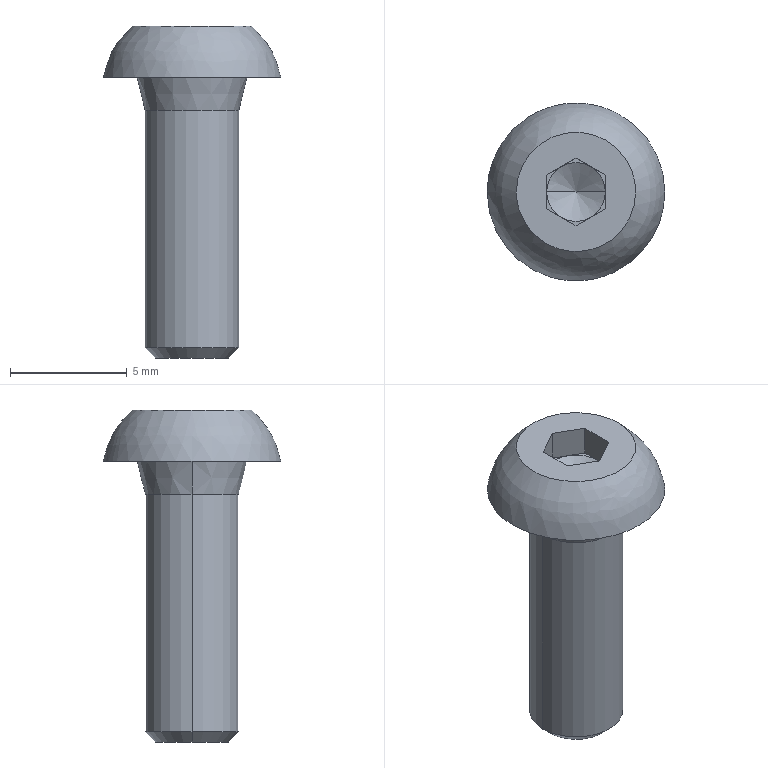Part | SolidWorks | features BaseBody 1 | 1 solid | 24 faces | box 7.6 x 7.6 x 14.2 mm | volume 222.779 mm3 | plane 15 | cone 6 | cylinder 2 | spline 1 | commonest cylinder face diameters 4 x2
STEP:
#1=CARTESIAN_POINT('',(2.,0.,-10.171));
#2=VERTEX_POINT('',#1);
#3=CARTESIAN_POINT('',(-2.,0.,-10.171));
#4=VERTEX_POINT('',#3);
#5=CARTESIAN_POINT('',(0.,0.,-10.171));
#6=DIRECTION('',(0.,0.,1.));
#7=DIRECTION('',(1.,0.,0.));
#8=AXIS2_PLACEMENT_3D('',#5,#6,#7);
#9=CIRCLE('',#8,2.);
#10=EDGE_CURVE('',#2,#4,#9,.T.);
#11=ORIENTED_EDGE('',*,*,#10,.T.);
#12=CARTESIAN_POINT('',(-2.,0.,0.));
#13=VERTEX_POINT('',#12);
#14=CARTESIAN_POINT('',(-2.,0.,-10.6));
#15=DIRECTION('',(0.,0.,1.));
#16=VECTOR('',#15,1000.);
#17=LINE('',#14,#16);
#18=EDGE_CURVE('',#4,#13,#17,.T.);
#19=ORIENTED_EDGE('',*,*,#18,.T.);
#20=CARTESIAN_POINT('',(2.,0.,0.));
#21=VERTEX_POINT('',#20);
#22=CARTESIAN_POINT('',(0.,0.,0.));
#23=DIRECTION('',(0.,0.,-1.));
#24=DIRECTION('',(1.,0.,0.));
#25=AXIS2_PLACEMENT_3D('',#22,#23,#24);
#26=CIRCLE('',#25,2.);
#27=EDGE_CURVE('',#13,#21,#26,.T.);
#28=ORIENTED_EDGE('',*,*,#27,.T.);
#29=CARTESIAN_POINT('',(2.,0.,-10.6));
#30=DIRECTION('',(0.,0.,1.));
#31=VECTOR('',#30,1000.);
#32=LINE('',#29,#31);
#33=EDGE_CURVE('',#2,#21,#32,.T.);
#34=ORIENTED_EDGE('',*,*,#33,.F.);
#35=EDGE_LOOP('',(#11,#19,#28,#34));
#36=FACE_OUTER_BOUND('',#35,.T.);
#37=CARTESIAN_POINT('',(0.,0.,-10.6));
#38=DIRECTION('',(0.,0.,1.));
#39=DIRECTION('',(1.,0.,0.));
#40=AXIS2_PLACEMENT_3D('',#37,#38,#39);
#41=CYLINDRICAL_SURFACE('',#40,2.);
#42=ADVANCED_FACE('',(#36),#41,.T.);
#43=ORIENTED_EDGE('',*,*,#27,.F.);
#44=CARTESIAN_POINT('',(-2.35,0.,1.4));
#45=VERTEX_POINT('',#44);
#46=CARTESIAN_POINT('',(-2.35,0.,1.4));
#47=DIRECTION('',(-0.2425,0.,0.9701));
#48=VECTOR('',#47,1000.);
#49=LINE('',#46,#48);
#50=EDGE_CURVE('',#13,#45,#49,.T.);
#51=ORIENTED_EDGE('',*,*,#50,.T.);
#52=CARTESIAN_POINT('',(2.35,0.,1.4));
#53=VERTEX_POINT('',#52);
#54=CARTESIAN_POINT('',(0.,0.,1.4));
#55=DIRECTION('',(0.,0.,-1.));
#56=DIRECTION('',(1.,0.,0.));
#57=AXIS2_PLACEMENT_3D('',#54,#55,#56);
#58=CIRCLE('',#57,2.35);
#59=EDGE_CURVE('',#45,#53,#58,.T.);
#60=ORIENTED_EDGE('',*,*,#59,.T.);
#61=CARTESIAN_POINT('',(2.35,0.,1.4));
#62=DIRECTION('',(0.2425,0.,0.9701));
#63=VECTOR('',#62,1000.);
#64=LINE('',#61,#63);
#65=EDGE_CURVE('',#21,#53,#64,.T.);
#66=ORIENTED_EDGE('',*,*,#65,.F.);
#67=EDGE_LOOP('',(#43,#51,#60,#66));
#68=FACE_OUTER_BOUND('',#67,.T.);
#69=CARTESIAN_POINT('',(0.,0.,1.4));
#70=DIRECTION('',(0.,0.,1.));
#71=DIRECTION('',(1.,0.,0.));
#72=AXIS2_PLACEMENT_3D('',#69,#70,#71);
#73=CONICAL_SURFACE('',#72,2.35,0.245);
#74=ADVANCED_FACE('',(#68),#73,.T.);
#75=CARTESIAN_POINT('',(1.571,0.,-10.6));
#76=VERTEX_POINT('',#75);
#77=CARTESIAN_POINT('',(-1.571,0.,-10.6));
#78=VERTEX_POINT('',#77);
#79=CARTESIAN_POINT('',(0.,0.,-10.6));
#80=DIRECTION('',(0.,0.,1.));
#81=DIRECTION('',(1.,0.,0.));
#82=AXIS2_PLACEMENT_3D('',#79,#80,#81);
#83=CIRCLE('',#82,1.571);
#84=EDGE_CURVE('',#76,#78,#83,.T.);
#85=ORIENTED_EDGE('',*,*,#84,.T.);
#86=CARTESIAN_POINT('',(-2.,0.,-10.171));
#87=DIRECTION('',(-0.7071,0.,0.7071));
#88=VECTOR('',#87,1000.);
#89=LINE('',#86,#88);
#90=EDGE_CURVE('',#78,#4,#89,.T.);
#91=ORIENTED_EDGE('',*,*,#90,.T.);
#92=ORIENTED_EDGE('',*,*,#10,.F.);
#93=CARTESIAN_POINT('',(2.,0.,-10.171));
#94=DIRECTION('',(0.7071,0.,0.7071));
#95=VECTOR('',#94,1000.);
#96=LINE('',#93,#95);
#97=EDGE_CURVE('',#76,#2,#96,.T.);
#98=ORIENTED_EDGE('',*,*,#97,.F.);
#99=EDGE_LOOP('',(#85,#91,#92,#98));
#100=FACE_OUTER_BOUND('',#99,.T.);
#101=CARTESIAN_POINT('',(0.,0.,-10.171));
#102=DIRECTION('',(0.,0.,1.));
#103=DIRECTION('',(1.,0.,0.));
#104=AXIS2_PLACEMENT_3D('',#101,#102,#103);
#105=CONICAL_SURFACE('',#104,2.,0.7854);
#106=ADVANCED_FACE('',(#100),#105,.T.);
#107=CARTESIAN_POINT('',(0.,0.,1.578));
#108=VERTEX_POINT('',#107);
#109=CARTESIAN_POINT('',(1.25,0.,2.3));
#110=VERTEX_POINT('',#109);
#111=CARTESIAN_POINT('',(1.25,0.,2.3));
#112=DIRECTION('',(0.866,0.,0.5));
#113=VECTOR('',#112,1000.);
#114=LINE('',#111,#113);
#115=EDGE_CURVE('',#108,#110,#114,.T.);
#116=ORIENTED_EDGE('',*,*,#115,.F.);
#117=CARTESIAN_POINT('',(-1.25,0.,2.3));
#118=VERTEX_POINT('',#117);
#119=CARTESIAN_POINT('',(-1.25,0.,2.3));
#120=DIRECTION('',(-0.866,0.,0.5));
#121=VECTOR('',#120,1000.);
#122=LINE('',#119,#121);
#123=EDGE_CURVE('',#108,#118,#122,.T.);
#124=ORIENTED_EDGE('',*,*,#123,.T.);
#125=CARTESIAN_POINT('',(-0.625,-1.083,2.3));
#126=VERTEX_POINT('',#125);
#127=CARTESIAN_POINT('',(0.,0.,2.3));
#128=DIRECTION('',(0.,0.,-1.));
#129=DIRECTION('',(1.,0.,0.));
#130=AXIS2_PLACEMENT_3D('',#127,#128,#129);
#131=CIRCLE('',#130,1.25);
#132=EDGE_CURVE('',#126,#118,#131,.T.);
#133=ORIENTED_EDGE('',*,*,#132,.F.);
#134=CARTESIAN_POINT('',(0.625,-1.083,2.3));
#135=VERTEX_POINT('',#134);
#136=CARTESIAN_POINT('',(0.,0.,2.3));
#137=DIRECTION('',(0.,0.,-1.));
#138=DIRECTION('',(1.,0.,0.));
#139=AXIS2_PLACEMENT_3D('',#136,#137,#138);
#140=CIRCLE('',#139,1.25);
#141=EDGE_CURVE('',#135,#126,#140,.T.);
#142=ORIENTED_EDGE('',*,*,#141,.F.);
#143=CARTESIAN_POINT('',(0.,0.,2.3));
#144=DIRECTION('',(0.,0.,-1.));
#145=DIRECTION('',(1.,0.,0.));
#146=AXIS2_PLACEMENT_3D('',#143,#144,#145);
#147=CIRCLE('',#146,1.25);
#148=EDGE_CURVE('',#110,#135,#147,.T.);
#149=ORIENTED_EDGE('',*,*,#148,.F.);
#150=EDGE_LOOP('',(#116,#124,#133,#142,#149));
#151=FACE_OUTER_BOUND('',#150,.T.);
#152=CARTESIAN_POINT('',(0.,0.,2.3));
#153=DIRECTION('',(0.,0.,1.));
#154=DIRECTION('',(1.,0.,0.));
#155=AXIS2_PLACEMENT_3D('',#152,#153,#154);
#156=CONICAL_SURFACE('',#155,1.25,1.047);
#157=ADVANCED_FACE('',(#151),#156,.F.);
#158=ORIENTED_EDGE('',*,*,#18,.F.);
#159=CARTESIAN_POINT('',(0.,0.,-10.171));
#160=DIRECTION('',(0.,0.,1.));
#161=DIRECTION('',(1.,0.,0.));
#162=AXIS2_PLACEMENT_3D('',#159,#160,#161);
#163=CIRCLE('',#162,2.);
#164=EDGE_CURVE('',#4,#2,#163,.T.);
#165=ORIENTED_EDGE('',*,*,#164,.T.);
#166=ORIENTED_EDGE('',*,*,#33,.T.);
#167=CARTESIAN_POINT('',(0.,0.,0.));
#168=DIRECTION('',(0.,0.,-1.));
#169=DIRECTION('',(1.,0.,0.));
#170=AXIS2_PLACEMENT_3D('',#167,#168,#169);
#171=CIRCLE('',#170,2.);
#172=EDGE_CURVE('',#21,#13,#171,.T.);
#173=ORIENTED_EDGE('',*,*,#172,.T.);
#174=EDGE_LOOP('',(#158,#165,#166,#173));
#175=FACE_OUTER_BOUND('',#174,.T.);
#176=CARTESIAN_POINT('',(0.,0.,-10.6));
#177=DIRECTION('',(0.,0.,1.));
#178=DIRECTION('',(1.,0.,0.));
#179=AXIS2_PLACEMENT_3D('',#176,#177,#178);
#180=CYLINDRICAL_SURFACE('',#179,2.);
#181=ADVANCED_FACE('',(#175),#180,.T.);
#182=ORIENTED_EDGE('',*,*,#50,.F.);
#183=ORIENTED_EDGE('',*,*,#172,.F.);
#184=ORIENTED_EDGE('',*,*,#65,.T.);
#185=CARTESIAN_POINT('',(0.,0.,1.4));
#186=DIRECTION('',(0.,0.,-1.));
#187=DIRECTION('',(1.,0.,0.));
#188=AXIS2_PLACEMENT_3D('',#185,#186,#187);
#189=CIRCLE('',#188,2.35);
#190=EDGE_CURVE('',#53,#45,#189,.T.);
#191=ORIENTED_EDGE('',*,*,#190,.T.);
#192=EDGE_LOOP('',(#182,#183,#184,#191));
#193=FACE_OUTER_BOUND('',#192,.T.);
#194=CARTESIAN_POINT('',(0.,0.,1.4));
#195=DIRECTION('',(0.,0.,1.));
#196=DIRECTION('',(1.,0.,0.));
#197=AXIS2_PLACEMENT_3D('',#194,#195,#196);
#198=CONICAL_SURFACE('',#197,2.35,0.245);
#199=ADVANCED_FACE('',(#193),#198,.T.);
#200=ORIENTED_EDGE('',*,*,#90,.F.);
#201=CARTESIAN_POINT('',(0.,0.,-10.6));
#202=DIRECTION('',(0.,0.,1.));
#203=DIRECTION('',(1.,0.,0.));
#204=AXIS2_PLACEMENT_3D('',#201,#202,#203);
#205=CIRCLE('',#204,1.571);
#206=EDGE_CURVE('',#78,#76,#205,.T.);
#207=ORIENTED_EDGE('',*,*,#206,.T.);
#208=ORIENTED_EDGE('',*,*,#97,.T.);
#209=ORIENTED_EDGE('',*,*,#164,.F.);
#210=EDGE_LOOP('',(#200,#207,#208,#209));
#211=FACE_OUTER_BOUND('',#210,.T.);
#212=CARTESIAN_POINT('',(0.,0.,-10.171));
#213=DIRECTION('',(0.,0.,1.));
#214=DIRECTION('',(1.,0.,0.));
#215=AXIS2_PLACEMENT_3D('',#212,#213,#214);
#216=CONICAL_SURFACE('',#215,2.,0.7854);
#217=ADVANCED_FACE('',(#211),#216,.T.);
#218=CARTESIAN_POINT('',(-3.8,0.,1.4));
#219=VERTEX_POINT('',#218);
#220=CARTESIAN_POINT('',(3.8,-0.001343,1.4));
#221=VERTEX_POINT('',#220);
#222=CARTESIAN_POINT('',(-3.8,0.,1.4));
#223=CARTESIAN_POINT('',(-3.8,-0.251,1.4));
#224=CARTESIAN_POINT('',(-3.775,-0.4979,1.4));
#225=CARTESIAN_POINT('',(-3.679,-0.9836,1.4));
#226=CARTESIAN_POINT('',(-3.606,-1.225,1.4));
#227=CARTESIAN_POINT('',(-3.415,-1.685,1.4));
#228=CARTESIAN_POINT('',(-3.298,-1.903,1.4));
#229=CARTESIAN_POINT('',(-3.023,-2.316,1.4));
#230=CARTESIAN_POINT('',(-2.862,-2.512,1.4));
#231=CARTESIAN_POINT('',(-2.511,-2.863,1.4));
#232=CARTESIAN_POINT('',(-2.32,-3.02,1.4));
#233=CARTESIAN_POINT('',(-1.905,-3.298,1.4));
#234=CARTESIAN_POINT('',(-1.684,-3.416,1.4));
#235=CARTESIAN_POINT('',(-1.226,-3.605,1.4));
#236=CARTESIAN_POINT('',(-0.9869,-3.678,1.4));
#237=CARTESIAN_POINT('',(-0.4964,-3.776,1.4));
#238=CARTESIAN_POINT('',(-0.2498,-3.8,1.4));
#239=CARTESIAN_POINT('',(0.2458,-3.8,1.4));
#240=CARTESIAN_POINT('',(0.4975,-3.775,1.4));
#241=CARTESIAN_POINT('',(0.9849,-3.679,1.4));
#242=CARTESIAN_POINT('',(1.222,-3.607,1.4));
#243=CARTESIAN_POINT('',(1.682,-3.417,1.4));
#244=CARTESIAN_POINT('',(1.904,-3.298,1.4));
#245=CARTESIAN_POINT('',(2.316,-3.023,1.4));
#246=CARTESIAN_POINT('',(2.508,-2.866,1.4));
#247=CARTESIAN_POINT('',(2.863,-2.511,1.4));
#248=CARTESIAN_POINT('',(3.021,-2.319,1.4));
#249=CARTESIAN_POINT('',(3.296,-1.907,1.4));
#250=CARTESIAN_POINT('',(3.415,-1.685,1.4));
#251=CARTESIAN_POINT('',(3.606,-1.225,1.4));
#252=CARTESIAN_POINT('',(3.678,-0.988,1.4));
#253=CARTESIAN_POINT('',(3.775,-0.5012,1.4));
#254=CARTESIAN_POINT('',(3.8,-0.2493,1.4));
#255=CARTESIAN_POINT('',(3.8,-0.001343,1.4));
#256=B_SPLINE_CURVE_WITH_KNOTS('',3,(#222,#223,#224,#225,#226,#227,#228,#229,#230,#231,#232,#233,#234,#235,#236,#237,#238,#239,#240,#241,#242,#243,#244,#245,#246,#247,#248,#249,#250,#251,#252,#253,#254,#255),.UNSPECIFIED.,.F.,.F.,(4,2,2,2,2,2,2,2,2,2,2,2,2,2,2,2,4),(0.,0.0007424,0.001485,0.002227,0.00297,0.003712,0.004455,0.005197,0.00594,0.006682,0.007424,0.008167,0.008909,0.009652,0.01039,0.01114,0.01188),.UNSPECIFIED.);
#257=EDGE_CURVE('',#219,#221,#256,.T.);
#258=ORIENTED_EDGE('',*,*,#257,.F.);
#259=CARTESIAN_POINT('',(3.8,-0.001343,1.4));
#260=CARTESIAN_POINT('',(3.8,0.2466,1.4));
#261=CARTESIAN_POINT('',(3.776,0.4931,1.4));
#262=CARTESIAN_POINT('',(3.679,0.9829,1.4));
#263=CARTESIAN_POINT('',(3.606,1.223,1.4));
#264=CARTESIAN_POINT('',(3.417,1.681,1.4));
#265=CARTESIAN_POINT('',(3.3,1.901,1.4));
#266=CARTESIAN_POINT('',(3.022,2.318,1.4));
#267=CARTESIAN_POINT('',(2.865,2.509,1.4));
#268=CARTESIAN_POINT('',(2.515,2.86,1.4));
#269=CARTESIAN_POINT('',(2.319,3.02,1.4));
#270=CARTESIAN_POINT('',(1.906,3.297,1.4));
#271=CARTESIAN_POINT('',(1.688,3.414,1.4));
#272=CARTESIAN_POINT('',(1.229,3.605,1.4));
#273=CARTESIAN_POINT('',(0.9869,3.678,1.4));
#274=CARTESIAN_POINT('',(0.5011,3.775,1.4));
#275=CARTESIAN_POINT('',(0.2544,3.8,1.4));
#276=CARTESIAN_POINT('',(-0.2467,3.8,1.4));
#277=CARTESIAN_POINT('',(-0.4947,3.776,1.4));
#278=CARTESIAN_POINT('',(-0.9803,3.68,1.4));
#279=CARTESIAN_POINT('',(-1.221,3.607,1.4));
#280=CARTESIAN_POINT('',(-1.682,3.417,1.4));
#281=CARTESIAN_POINT('',(-1.901,3.3,1.4));
#282=CARTESIAN_POINT('',(-2.313,3.025,1.4));
#283=CARTESIAN_POINT('',(-2.509,2.864,1.4));
#284=CARTESIAN_POINT('',(-2.86,2.514,1.4));
#285=CARTESIAN_POINT('',(-3.018,2.323,1.4));
#286=CARTESIAN_POINT('',(-3.296,1.908,1.4));
#287=CARTESIAN_POINT('',(-3.414,1.687,1.4));
#288=CARTESIAN_POINT('',(-3.604,1.229,1.4));
#289=CARTESIAN_POINT('',(-3.677,0.9912,1.4));
#290=CARTESIAN_POINT('',(-3.775,0.4995,1.4));
#291=CARTESIAN_POINT('',(-3.8,0.251,1.4));
#292=CARTESIAN_POINT('',(-3.8,0.,1.4));
#293=B_SPLINE_CURVE_WITH_KNOTS('',3,(#259,#260,#261,#262,#263,#264,#265,#266,#267,#268,#269,#270,#271,#272,#273,#274,#275,#276,#277,#278,#279,#280,#281,#282,#283,#284,#285,#286,#287,#288,#289,#290,#291,#292),.UNSPECIFIED.,.F.,.F.,(4,2,2,2,2,2,2,2,2,2,2,2,2,2,2,2,4),(0.01188,0.01262,0.01336,0.01411,0.01485,0.01559,0.01633,0.01708,0.01782,0.01856,0.0193,0.02005,0.02079,0.02153,0.02227,0.02302,0.02376),.UNSPECIFIED.);
#294=EDGE_CURVE('',#221,#219,#293,.T.);
#295=ORIENTED_EDGE('',*,*,#294,.F.);
#296=EDGE_LOOP('',(#258,#295));
#297=FACE_OUTER_BOUND('',#296,.T.);
#298=ORIENTED_EDGE('',*,*,#190,.F.);
#299=ORIENTED_EDGE('',*,*,#59,.F.);
#300=EDGE_LOOP('',(#298,#299));
#301=FACE_BOUND('',#300,.T.);
#302=CARTESIAN_POINT('',(0.,3.8,1.4));
#303=DIRECTION('',(0.,0.,1.));
#304=DIRECTION('',(1.,0.,0.));
#305=AXIS2_PLACEMENT_3D('',#302,#303,#304);
#306=PLANE('',#305);
#307=ADVANCED_FACE('',(#297,#301),#306,.F.);
#308=ORIENTED_EDGE('',*,*,#84,.F.);
#309=ORIENTED_EDGE('',*,*,#206,.F.);
#310=EDGE_LOOP('',(#308,#309));
#311=FACE_OUTER_BOUND('',#310,.T.);
#312=CARTESIAN_POINT('',(0.,1.571,-10.6));
#313=DIRECTION('',(0.,0.,1.));
#314=DIRECTION('',(1.,0.,0.));
#315=AXIS2_PLACEMENT_3D('',#312,#313,#314);
#316=PLANE('',#315);
#317=ADVANCED_FACE('',(#311),#316,.F.);
#318=ORIENTED_EDGE('',*,*,#257,.T.);
#319=ORIENTED_EDGE('',*,*,#294,.T.);
#320=EDGE_LOOP('',(#318,#319));
#321=FACE_OUTER_BOUND('',#320,.T.);
#322=CARTESIAN_POINT('',(-2.553,0.,3.6));
#323=VERTEX_POINT('',#322);
#324=CARTESIAN_POINT('',(2.553,0.0009026,3.6));
#325=VERTEX_POINT('',#324);
#326=CARTESIAN_POINT('',(-2.553,0.,3.6));
#327=CARTESIAN_POINT('',(-2.553,0.1687,3.6));
#328=CARTESIAN_POINT('',(-2.537,0.3346,3.6));
#329=CARTESIAN_POINT('',(-2.472,0.6609,3.6));
#330=CARTESIAN_POINT('',(-2.423,0.8231,3.6));
#331=CARTESIAN_POINT('',(-2.295,1.132,3.6));
#332=CARTESIAN_POINT('',(-2.216,1.279,3.6));
#333=CARTESIAN_POINT('',(-2.031,1.557,3.6));
#334=CARTESIAN_POINT('',(-1.923,1.688,3.6));
#335=CARTESIAN_POINT('',(-1.688,1.923,3.6));
#336=CARTESIAN_POINT('',(-1.559,2.029,3.6));
#337=CARTESIAN_POINT('',(-1.28,2.216,3.6));
#338=CARTESIAN_POINT('',(-1.131,2.295,3.6));
#339=CARTESIAN_POINT('',(-0.824,2.423,3.6));
#340=CARTESIAN_POINT('',(-0.6632,2.472,3.6));
#341=CARTESIAN_POINT('',(-0.3336,2.537,3.6));
#342=CARTESIAN_POINT('',(-0.1679,2.553,3.6));
#343=CARTESIAN_POINT('',(0.1652,2.554,3.6));
#344=CARTESIAN_POINT('',(0.3343,2.537,3.6));
#345=CARTESIAN_POINT('',(0.6618,2.472,3.6));
#346=CARTESIAN_POINT('',(0.821,2.424,3.6));
#347=CARTESIAN_POINT('',(1.13,2.296,3.6));
#348=CARTESIAN_POINT('',(1.28,2.216,3.6));
#349=CARTESIAN_POINT('',(1.556,2.031,3.6));
#350=CARTESIAN_POINT('',(1.685,1.926,3.6));
#351=CARTESIAN_POINT('',(1.924,1.687,3.6));
#352=CARTESIAN_POINT('',(2.03,1.558,3.6));
#353=CARTESIAN_POINT('',(2.215,1.282,3.6));
#354=CARTESIAN_POINT('',(2.295,1.132,3.6));
#355=CARTESIAN_POINT('',(2.423,0.823,3.6));
#356=CARTESIAN_POINT('',(2.471,0.6639,3.6));
#357=CARTESIAN_POINT('',(2.537,0.3368,3.6));
#358=CARTESIAN_POINT('',(2.553,0.1675,3.6));
#359=CARTESIAN_POINT('',(2.553,0.0009026,3.6));
#360=B_SPLINE_CURVE_WITH_KNOTS('',3,(#326,#327,#328,#329,#330,#331,#332,#333,#334,#335,#336,#337,#338,#339,#340,#341,#342,#343,#344,#345,#346,#347,#348,#349,#350,#351,#352,#353,#354,#355,#356,#357,#358,#359),.UNSPECIFIED.,.F.,.F.,(4,2,2,2,2,2,2,2,2,2,2,2,2,2,2,2,4),(0.,0.0004989,0.0009978,0.001497,0.001996,0.002494,0.002993,0.003492,0.003991,0.00449,0.004989,0.005488,0.005987,0.006486,0.006985,0.007483,0.007982),.UNSPECIFIED.);
#361=EDGE_CURVE('',#323,#325,#360,.T.);
#362=ORIENTED_EDGE('',*,*,#361,.T.);
#363=CARTESIAN_POINT('',(2.553,0.0009026,3.6));
#364=CARTESIAN_POINT('',(2.553,-0.1657,3.6));
#365=CARTESIAN_POINT('',(2.537,-0.3313,3.6));
#366=CARTESIAN_POINT('',(2.472,-0.6605,3.6));
#367=CARTESIAN_POINT('',(2.423,-0.8219,3.6));
#368=CARTESIAN_POINT('',(2.233,-1.283,3.6));
#369=CARTESIAN_POINT('',(2.043,-1.568,3.6));
#370=CARTESIAN_POINT('',(1.69,-1.922,3.6));
#371=CARTESIAN_POINT('',(1.559,-2.03,3.6));
#372=CARTESIAN_POINT('',(1.281,-2.215,3.6));
#373=CARTESIAN_POINT('',(1.134,-2.294,3.6));
#374=CARTESIAN_POINT('',(0.8255,-2.422,3.6));
#375=CARTESIAN_POINT('',(0.6631,-2.471,3.6));
#376=CARTESIAN_POINT('',(0.3367,-2.537,3.6));
#377=CARTESIAN_POINT('',(0.171,-2.553,3.6));
#378=CARTESIAN_POINT('',(-0.1658,-2.554,3.6));
#379=CARTESIAN_POINT('',(-0.3324,-2.537,3.6));
#380=CARTESIAN_POINT('',(-0.6587,-2.473,3.6));
#381=CARTESIAN_POINT('',(-0.8205,-2.424,3.6));
#382=CARTESIAN_POINT('',(-1.13,-2.296,3.6));
#383=CARTESIAN_POINT('',(-1.277,-2.217,3.6));
#384=CARTESIAN_POINT('',(-1.555,-2.033,3.6));
#385=CARTESIAN_POINT('',(-1.686,-1.925,3.6));
#386=CARTESIAN_POINT('',(-1.922,-1.689,3.6));
#387=CARTESIAN_POINT('',(-2.028,-1.561,3.6));
#388=CARTESIAN_POINT('',(-2.214,-1.282,3.6));
#389=CARTESIAN_POINT('',(-2.294,-1.133,3.6));
#390=CARTESIAN_POINT('',(-2.486,-0.6725,3.6));
#391=CARTESIAN_POINT('',(-2.553,-0.3374,3.6));
#392=CARTESIAN_POINT('',(-2.553,0.,3.6));
#393=B_SPLINE_CURVE_WITH_KNOTS('',3,(#363,#364,#365,#366,#367,#368,#369,#370,#371,#372,#373,#374,#375,#376,#377,#378,#379,#380,#381,#382,#383,#384,#385,#386,#387,#388,#389,#390,#391,#392),.UNSPECIFIED.,.F.,.F.,(4,2,2,2,2,2,2,2,2,2,2,2,2,2,4),(0.007982,0.008481,0.00898,0.009978,0.01048,0.01098,0.01147,0.01197,0.01247,0.01297,0.01347,0.01397,0.01447,0.01497,0.01596),.UNSPECIFIED.);
#394=EDGE_CURVE('',#325,#323,#393,.T.);
#395=ORIENTED_EDGE('',*,*,#394,.T.);
#396=EDGE_LOOP('',(#362,#395));
#397=FACE_BOUND('',#396,.T.);
#398=CARTESIAN_POINT('',(-0.6038,3.815,0.8008));
#399=CARTESIAN_POINT('',(-0.454,3.815,1.698));
#400=CARTESIAN_POINT('',(0.4551,3.815,1.697));
#401=CARTESIAN_POINT('',(0.6039,3.815,0.8002));
#402=CARTESIAN_POINT('',(-6.341,2.882,1.759));
#403=CARTESIAN_POINT('',(-4.768,2.882,11.177));
#404=CARTESIAN_POINT('',(4.78,2.882,11.171));
#405=CARTESIAN_POINT('',(6.342,2.882,1.752));
#406=CARTESIAN_POINT('',(-6.283,-3.009,1.749));
#407=CARTESIAN_POINT('',(-4.725,-3.009,11.081));
#408=CARTESIAN_POINT('',(4.736,-3.009,11.076));
#409=CARTESIAN_POINT('',(6.285,-3.009,1.742));
#410=CARTESIAN_POINT('',(-0.5289,-3.827,0.7883));
#411=CARTESIAN_POINT('',(-0.3977,-3.827,1.574));
#412=CARTESIAN_POINT('',(0.3987,-3.827,1.573));
#413=CARTESIAN_POINT('',(0.529,-3.827,0.7877));
#414=(BOUNDED_SURFACE()B_SPLINE_SURFACE(3,3,((#398,#399,#400,#401),(#402,#403,#404,#405),(#406,#407,#408,#409),(#410,#411,#412,#413)),.UNSPECIFIED.,.F.,.F.,.F.)B_SPLINE_SURFACE_WITH_KNOTS((4,4),(4,4),(0.,1.),(0.,1.),.UNSPECIFIED.)GEOMETRIC_REPRESENTATION_ITEM()RATIONAL_B_SPLINE_SURFACE(((1.,0.4428,0.4428,1.),(0.4324,0.1915,0.1915,0.4324),(0.4324,0.1915,0.1915,0.4324),(1.,0.4428,0.4428,1.)))REPRESENTATION_ITEM('')SURFACE());
#415=ADVANCED_FACE('',(#321,#397),#414,.T.);
#416=CARTESIAN_POINT('',(-1.25,-0.7217,3.6));
#417=VERTEX_POINT('',#416);
#418=CARTESIAN_POINT('',(0.,-1.443,3.6));
#419=VERTEX_POINT('',#418);
#420=CARTESIAN_POINT('',(-1.25,-0.7217,3.6));
#421=DIRECTION('',(0.866,-0.5,0.));
#422=VECTOR('',#421,1000.);
#423=LINE('',#420,#422);
#424=EDGE_CURVE('',#417,#419,#423,.T.);
#425=ORIENTED_EDGE('',*,*,#424,.F.);
#426=CARTESIAN_POINT('',(-1.25,0.7217,3.6));
#427=VERTEX_POINT('',#426);
#428=CARTESIAN_POINT('',(-1.25,0.,3.6));
#429=DIRECTION('',(0.,-1.,0.));
#430=VECTOR('',#429,1000.);
#431=LINE('',#428,#430);
#432=EDGE_CURVE('',#427,#417,#431,.T.);
#433=ORIENTED_EDGE('',*,*,#432,.F.);
#434=CARTESIAN_POINT('',(0.,1.443,3.6));
#435=VERTEX_POINT('',#434);
#436=CARTESIAN_POINT('',(0.,1.443,3.6));
#437=DIRECTION('',(-0.866,-0.5,0.));
#438=VECTOR('',#437,1000.);
#439=LINE('',#436,#438);
#440=EDGE_CURVE('',#435,#427,#439,.T.);
#441=ORIENTED_EDGE('',*,*,#440,.F.);
#442=CARTESIAN_POINT('',(1.25,0.7217,3.6));
#443=VERTEX_POINT('',#442);
#444=CARTESIAN_POINT('',(1.25,0.7217,3.6));
#445=DIRECTION('',(-0.866,0.5,0.));
#446=VECTOR('',#445,1000.);
#447=LINE('',#444,#446);
#448=EDGE_CURVE('',#443,#435,#447,.T.);
#449=ORIENTED_EDGE('',*,*,#448,.F.);
#450=CARTESIAN_POINT('',(1.25,-0.7217,3.6));
#451=VERTEX_POINT('',#450);
#452=CARTESIAN_POINT('',(1.25,0.,3.6));
#453=DIRECTION('',(0.,1.,0.));
#454=VECTOR('',#453,1000.);
#455=LINE('',#452,#454);
#456=EDGE_CURVE('',#451,#443,#455,.T.);
#457=ORIENTED_EDGE('',*,*,#456,.F.);
#458=CARTESIAN_POINT('',(0.,-1.443,3.6));
#459=DIRECTION('',(0.866,0.5,0.));
#460=VECTOR('',#459,1000.);
#461=LINE('',#458,#460);
#462=EDGE_CURVE('',#419,#451,#461,.T.);
#463=ORIENTED_EDGE('',*,*,#462,.F.);
#464=EDGE_LOOP('',(#425,#433,#441,#449,#457,#463));
#465=FACE_BOUND('',#464,.T.);
#466=ORIENTED_EDGE('',*,*,#361,.F.);
#467=ORIENTED_EDGE('',*,*,#394,.F.);
#468=EDGE_LOOP('',(#466,#467));
#469=FACE_OUTER_BOUND('',#468,.T.);
#470=CARTESIAN_POINT('',(0.,0.,3.6));
#471=DIRECTION('',(0.,0.,-1.));
#472=DIRECTION('',(-1.,0.,0.));
#473=AXIS2_PLACEMENT_3D('',#470,#471,#472);
#474=PLANE('',#473);
#475=ADVANCED_FACE('',(#465,#469),#474,.F.);
#476=CARTESIAN_POINT('',(1.25,-0.7217,2.3));
#477=VERTEX_POINT('',#476);
#478=CARTESIAN_POINT('',(1.25,-0.7217,2.3));
#479=DIRECTION('',(0.,0.,1.));
#480=VECTOR('',#479,1000.);
#481=LINE('',#478,#480);
#482=EDGE_CURVE('',#477,#451,#481,.T.);
#483=ORIENTED_EDGE('',*,*,#482,.F.);
#484=CARTESIAN_POINT('',(0.,-1.443,2.3));
#485=DIRECTION('',(0.866,0.5,0.));
#486=VECTOR('',#485,1000.);
#487=LINE('',#484,#486);
#488=EDGE_CURVE('',#135,#477,#487,.T.);
#489=ORIENTED_EDGE('',*,*,#488,.F.);
#490=CARTESIAN_POINT('',(0.,-1.443,2.3));
#491=VERTEX_POINT('',#490);
#492=CARTESIAN_POINT('',(0.,-1.443,2.3));
#493=DIRECTION('',(0.866,0.5,0.));
#494=VECTOR('',#493,1000.);
#495=LINE('',#492,#494);
#496=EDGE_CURVE('',#491,#135,#495,.T.);
#497=ORIENTED_EDGE('',*,*,#496,.F.);
#498=CARTESIAN_POINT('',(0.,-1.443,2.3));
#499=DIRECTION('',(0.,0.,-1.));
#500=VECTOR('',#499,1000.);
#501=LINE('',#498,#500);
#502=EDGE_CURVE('',#419,#491,#501,.T.);
#503=ORIENTED_EDGE('',*,*,#502,.F.);
#504=ORIENTED_EDGE('',*,*,#462,.T.);
#505=EDGE_LOOP('',(#483,#489,#497,#503,#504));
#506=FACE_OUTER_BOUND('',#505,.T.);
#507=CARTESIAN_POINT('',(0.,-1.443,2.3));
#508=DIRECTION('',(0.5,-0.866,0.));
#509=DIRECTION('',(0.866,0.5,0.));
#510=AXIS2_PLACEMENT_3D('',#507,#508,#509);
#511=PLANE('',#510);
#512=ADVANCED_FACE('',(#506),#511,.F.);
#513=ORIENTED_EDGE('',*,*,#502,.T.);
#514=CARTESIAN_POINT('',(-1.25,-0.7217,2.3));
#515=DIRECTION('',(0.866,-0.5,0.));
#516=VECTOR('',#515,1000.);
#517=LINE('',#514,#516);
#518=EDGE_CURVE('',#126,#491,#517,.T.);
#519=ORIENTED_EDGE('',*,*,#518,.F.);
#520=CARTESIAN_POINT('',(-1.25,-0.7217,2.3));
#521=VERTEX_POINT('',#520);
#522=CARTESIAN_POINT('',(-1.25,-0.7217,2.3));
#523=DIRECTION('',(0.866,-0.5,0.));
#524=VECTOR('',#523,1000.);
#525=LINE('',#522,#524);
#526=EDGE_CURVE('',#521,#126,#525,.T.);
#527=ORIENTED_EDGE('',*,*,#526,.F.);
#528=CARTESIAN_POINT('',(-1.25,-0.7217,2.3));
#529=DIRECTION('',(0.,0.,-1.));
#530=VECTOR('',#529,1000.);
#531=LINE('',#528,#530);
#532=EDGE_CURVE('',#417,#521,#531,.T.);
#533=ORIENTED_EDGE('',*,*,#532,.F.);
#534=ORIENTED_EDGE('',*,*,#424,.T.);
#535=EDGE_LOOP('',(#513,#519,#527,#533,#534));
#536=FACE_OUTER_BOUND('',#535,.T.);
#537=CARTESIAN_POINT('',(-1.25,-0.7217,2.3));
#538=DIRECTION('',(-0.5,-0.866,0.));
#539=DIRECTION('',(0.866,-0.5,0.));
#540=AXIS2_PLACEMENT_3D('',#537,#538,#539);
#541=PLANE('',#540);
#542=ADVANCED_FACE('',(#536),#541,.F.);
#543=ORIENTED_EDGE('',*,*,#532,.T.);
#544=CARTESIAN_POINT('',(-1.25,0.7217,2.3));
#545=DIRECTION('',(0.,-1.,0.));
#546=VECTOR('',#545,1000.);
#547=LINE('',#544,#546);
#548=EDGE_CURVE('',#118,#521,#547,.T.);
#549=ORIENTED_EDGE('',*,*,#548,.F.);
#550=CARTESIAN_POINT('',(-1.25,0.7217,2.3));
#551=VERTEX_POINT('',#550);
#552=CARTESIAN_POINT('',(-1.25,0.7217,2.3));
#553=DIRECTION('',(0.,-1.,0.));
#554=VECTOR('',#553,1000.);
#555=LINE('',#552,#554);
#556=EDGE_CURVE('',#551,#118,#555,.T.);
#557=ORIENTED_EDGE('',*,*,#556,.F.);
#558=CARTESIAN_POINT('',(-1.25,0.7217,2.3));
#559=DIRECTION('',(0.,0.,-1.));
#560=VECTOR('',#559,1000.);
#561=LINE('',#558,#560);
#562=EDGE_CURVE('',#427,#551,#561,.T.);
#563=ORIENTED_EDGE('',*,*,#562,.F.);
#564=ORIENTED_EDGE('',*,*,#432,.T.);
#565=EDGE_LOOP('',(#543,#549,#557,#563,#564));
#566=FACE_OUTER_BOUND('',#565,.T.);
#567=CARTESIAN_POINT('',(-1.25,0.7217,2.3));
#568=DIRECTION('',(-1.,0.,0.));
#569=DIRECTION('',(0.,0.,1.));
#570=AXIS2_PLACEMENT_3D('',#567,#568,#569);
#571=PLANE('',#570);
#572=ADVANCED_FACE('',(#566),#571,.F.);
#573=ORIENTED_EDGE('',*,*,#562,.T.);
#574=CARTESIAN_POINT('',(-0.625,1.083,2.3));
#575=VERTEX_POINT('',#574);
#576=CARTESIAN_POINT('',(0.,1.443,2.3));
#577=DIRECTION('',(-0.866,-0.5,0.));
#578=VECTOR('',#577,1000.);
#579=LINE('',#576,#578);
#580=EDGE_CURVE('',#575,#551,#579,.T.);
#581=ORIENTED_EDGE('',*,*,#580,.F.);
#582=CARTESIAN_POINT('',(0.,1.443,2.3));
#583=VERTEX_POINT('',#582);
#584=CARTESIAN_POINT('',(0.,1.443,2.3));
#585=DIRECTION('',(-0.866,-0.5,0.));
#586=VECTOR('',#585,1000.);
#587=LINE('',#584,#586);
#588=EDGE_CURVE('',#583,#575,#587,.T.);
#589=ORIENTED_EDGE('',*,*,#588,.F.);
#590=CARTESIAN_POINT('',(0.,1.443,2.3));
#591=DIRECTION('',(0.,0.,-1.));
#592=VECTOR('',#591,1000.);
#593=LINE('',#590,#592);
#594=EDGE_CURVE('',#435,#583,#593,.T.);
#595=ORIENTED_EDGE('',*,*,#594,.F.);
#596=ORIENTED_EDGE('',*,*,#440,.T.);
#597=EDGE_LOOP('',(#573,#581,#589,#595,#596));
#598=FACE_OUTER_BOUND('',#597,.T.);
#599=CARTESIAN_POINT('',(0.,1.443,2.3));
#600=DIRECTION('',(-0.5,0.866,0.));
#601=DIRECTION('',(-0.866,-0.5,0.));
#602=AXIS2_PLACEMENT_3D('',#599,#600,#601);
#603=PLANE('',#602);
#604=ADVANCED_FACE('',(#598),#603,.F.);
#605=ORIENTED_EDGE('',*,*,#594,.T.);
#606=CARTESIAN_POINT('',(0.625,1.083,2.3));
#607=VERTEX_POINT('',#606);
#608=CARTESIAN_POINT('',(1.25,0.7217,2.3));
#609=DIRECTION('',(-0.866,0.5,0.));
#610=VECTOR('',#609,1000.);
#611=LINE('',#608,#610);
#612=EDGE_CURVE('',#607,#583,#611,.T.);
#613=ORIENTED_EDGE('',*,*,#612,.F.);
#614=CARTESIAN_POINT('',(1.25,0.7217,2.3));
#615=VERTEX_POINT('',#614);
#616=CARTESIAN_POINT('',(1.25,0.7217,2.3));
#617=DIRECTION('',(-0.866,0.5,0.));
#618=VECTOR('',#617,1000.);
#619=LINE('',#616,#618);
#620=EDGE_CURVE('',#615,#607,#619,.T.);
#621=ORIENTED_EDGE('',*,*,#620,.F.);
#622=CARTESIAN_POINT('',(1.25,0.7217,2.3));
#623=DIRECTION('',(0.,0.,-1.));
#624=VECTOR('',#623,1000.);
#625=LINE('',#622,#624);
#626=EDGE_CURVE('',#443,#615,#625,.T.);
#627=ORIENTED_EDGE('',*,*,#626,.F.);
#628=ORIENTED_EDGE('',*,*,#448,.T.);
#629=EDGE_LOOP('',(#605,#613,#621,#627,#628));
#630=FACE_OUTER_BOUND('',#629,.T.);
#631=CARTESIAN_POINT('',(1.25,0.7217,2.3));
#632=DIRECTION('',(0.5,0.866,0.));
#633=DIRECTION('',(-0.866,0.5,0.));
#634=AXIS2_PLACEMENT_3D('',#631,#632,#633);
#635=PLANE('',#634);
#636=ADVANCED_FACE('',(#630),#635,.F.);
#637=ORIENTED_EDGE('',*,*,#626,.T.);
#638=CARTESIAN_POINT('',(1.25,-0.7217,2.3));
#639=DIRECTION('',(0.,1.,0.));
#640=VECTOR('',#639,1000.);
#641=LINE('',#638,#640);
#642=EDGE_CURVE('',#110,#615,#641,.T.);
#643=ORIENTED_EDGE('',*,*,#642,.F.);
#644=CARTESIAN_POINT('',(1.25,-0.7217,2.3));
#645=DIRECTION('',(0.,1.,0.));
#646=VECTOR('',#645,1000.);
#647=LINE('',#644,#646);
#648=EDGE_CURVE('',#477,#110,#647,.T.);
#649=ORIENTED_EDGE('',*,*,#648,.F.);
#650=ORIENTED_EDGE('',*,*,#482,.T.);
#651=ORIENTED_EDGE('',*,*,#456,.T.);
#652=EDGE_LOOP('',(#637,#643,#649,#650,#651));
#653=FACE_OUTER_BOUND('',#652,.T.);
#654=CARTESIAN_POINT('',(1.25,-0.7217,2.3));
#655=DIRECTION('',(1.,0.,0.));
#656=DIRECTION('',(0.,0.,-1.));
#657=AXIS2_PLACEMENT_3D('',#654,#655,#656);
#658=PLANE('',#657);
#659=ADVANCED_FACE('',(#653),#658,.F.);
#660=ORIENTED_EDGE('',*,*,#148,.T.);
#661=ORIENTED_EDGE('',*,*,#488,.T.);
#662=ORIENTED_EDGE('',*,*,#648,.T.);
#663=EDGE_LOOP('',(#660,#661,#662));
#664=FACE_OUTER_BOUND('',#663,.T.);
#665=CARTESIAN_POINT('',(0.,0.,2.3));
#666=DIRECTION('',(0.,0.,1.));
#667=DIRECTION('',(1.,0.,0.));
#668=AXIS2_PLACEMENT_3D('',#665,#666,#667);
#669=PLANE('',#668);
#670=ADVANCED_FACE('',(#664),#669,.T.);
#671=ORIENTED_EDGE('',*,*,#141,.T.);
#672=ORIENTED_EDGE('',*,*,#518,.T.);
#673=ORIENTED_EDGE('',*,*,#496,.T.);
#674=EDGE_LOOP('',(#671,#672,#673));
#675=FACE_OUTER_BOUND('',#674,.T.);
#676=CARTESIAN_POINT('',(0.,0.,2.3));
#677=DIRECTION('',(0.,0.,1.));
#678=DIRECTION('',(1.,0.,0.));
#679=AXIS2_PLACEMENT_3D('',#676,#677,#678);
#680=PLANE('',#679);
#681=ADVANCED_FACE('',(#675),#680,.T.);
#682=ORIENTED_EDGE('',*,*,#132,.T.);
#683=ORIENTED_EDGE('',*,*,#548,.T.);
#684=ORIENTED_EDGE('',*,*,#526,.T.);
#685=EDGE_LOOP('',(#682,#683,#684));
#686=FACE_OUTER_BOUND('',#685,.T.);
#687=CARTESIAN_POINT('',(0.,0.,2.3));
#688=DIRECTION('',(0.,0.,1.));
#689=DIRECTION('',(1.,0.,0.));
#690=AXIS2_PLACEMENT_3D('',#687,#688,#689);
#691=PLANE('',#690);
#692=ADVANCED_FACE('',(#686),#691,.T.);
#693=CARTESIAN_POINT('',(0.,0.,2.3));
#694=DIRECTION('',(0.,0.,-1.));
#695=DIRECTION('',(1.,0.,0.));
#696=AXIS2_PLACEMENT_3D('',#693,#694,#695);
#697=CIRCLE('',#696,1.25);
#698=EDGE_CURVE('',#118,#575,#697,.T.);
#699=ORIENTED_EDGE('',*,*,#698,.T.);
#700=ORIENTED_EDGE('',*,*,#580,.T.);
#701=ORIENTED_EDGE('',*,*,#556,.T.);
#702=EDGE_LOOP('',(#699,#700,#701));
#703=FACE_OUTER_BOUND('',#702,.T.);
#704=CARTESIAN_POINT('',(0.,0.,2.3));
#705=DIRECTION('',(0.,0.,1.));
#706=DIRECTION('',(1.,0.,0.));
#707=AXIS2_PLACEMENT_3D('',#704,#705,#706);
#708=PLANE('',#707);
#709=ADVANCED_FACE('',(#703),#708,.T.);
#710=CARTESIAN_POINT('',(0.,0.,2.3));
#711=DIRECTION('',(0.,0.,-1.));
#712=DIRECTION('',(1.,0.,0.));
#713=AXIS2_PLACEMENT_3D('',#710,#711,#712);
#714=CIRCLE('',#713,1.25);
#715=EDGE_CURVE('',#575,#607,#714,.T.);
#716=ORIENTED_EDGE('',*,*,#715,.T.);
#717=ORIENTED_EDGE('',*,*,#612,.T.);
#718=ORIENTED_EDGE('',*,*,#588,.T.);
#719=EDGE_LOOP('',(#716,#717,#718));
#720=FACE_OUTER_BOUND('',#719,.T.);
#721=CARTESIAN_POINT('',(0.,0.,2.3));
#722=DIRECTION('',(0.,0.,1.));
#723=DIRECTION('',(1.,0.,0.));
#724=AXIS2_PLACEMENT_3D('',#721,#722,#723);
#725=PLANE('',#724);
#726=ADVANCED_FACE('',(#720),#725,.T.);
#727=CARTESIAN_POINT('',(0.,0.,2.3));
#728=DIRECTION('',(0.,0.,-1.));
#729=DIRECTION('',(1.,0.,0.));
#730=AXIS2_PLACEMENT_3D('',#727,#728,#729);
#731=CIRCLE('',#730,1.25);
#732=EDGE_CURVE('',#607,#110,#731,.T.);
#733=ORIENTED_EDGE('',*,*,#732,.T.);
#734=ORIENTED_EDGE('',*,*,#642,.T.);
#735=ORIENTED_EDGE('',*,*,#620,.T.);
#736=EDGE_LOOP('',(#733,#734,#735));
#737=FACE_OUTER_BOUND('',#736,.T.);
#738=CARTESIAN_POINT('',(0.,0.,2.3));
#739=DIRECTION('',(0.,0.,1.));
#740=DIRECTION('',(1.,0.,0.));
#741=AXIS2_PLACEMENT_3D('',#738,#739,#740);
#742=PLANE('',#741);
#743=ADVANCED_FACE('',(#737),#742,.T.);
#744=ORIENTED_EDGE('',*,*,#123,.F.);
#745=ORIENTED_EDGE('',*,*,#115,.T.);
#746=ORIENTED_EDGE('',*,*,#732,.F.);
#747=ORIENTED_EDGE('',*,*,#715,.F.);
#748=ORIENTED_EDGE('',*,*,#698,.F.);
#749=EDGE_LOOP('',(#744,#745,#746,#747,#748));
#750=FACE_OUTER_BOUND('',#749,.T.);
#751=CARTESIAN_POINT('',(0.,0.,2.3));
#752=DIRECTION('',(0.,0.,1.));
#753=DIRECTION('',(1.,0.,0.));
#754=AXIS2_PLACEMENT_3D('',#751,#752,#753);
#755=CONICAL_SURFACE('',#754,1.25,1.047);
#756=ADVANCED_FACE('',(#750),#755,.F.);
#757=CLOSED_SHELL('',(#42,#74,#106,#157,#181,#199,#217,#307,#317,#415,#475,#512,#542,#572,#604,#636,#659,#670,#681,#692,#709,#726,#743,#756));
#758=MANIFOLD_SOLID_BREP('',#757);
#759=CARTESIAN_POINT('',(0.,0.,0.));
#760=DIRECTION('',(0.,0.,1.));
#761=DIRECTION('',(1.,0.,0.));
#762=AXIS2_PLACEMENT_3D('',#759,#760,#761);
#763=(LENGTH_UNIT()NAMED_UNIT(*)SI_UNIT(.MILLI.,.METRE.));
#764=UNCERTAINTY_MEASURE_WITH_UNIT(LENGTH_MEASURE(0.00001),#763,'','');
#765=(NAMED_UNIT(*)PLANE_ANGLE_UNIT()SI_UNIT($,.RADIAN.));
#766=(NAMED_UNIT(*)SI_UNIT($,.STERADIAN.)SOLID_ANGLE_UNIT());
#767=(GEOMETRIC_REPRESENTATION_CONTEXT(3)GLOBAL_UNCERTAINTY_ASSIGNED_CONTEXT((#764))GLOBAL_UNIT_ASSIGNED_CONTEXT((#763,#765,#766))REPRESENTATION_CONTEXT('',''));
#768=ADVANCED_BREP_SHAPE_REPRESENTATION('',(#758,#762),#767);